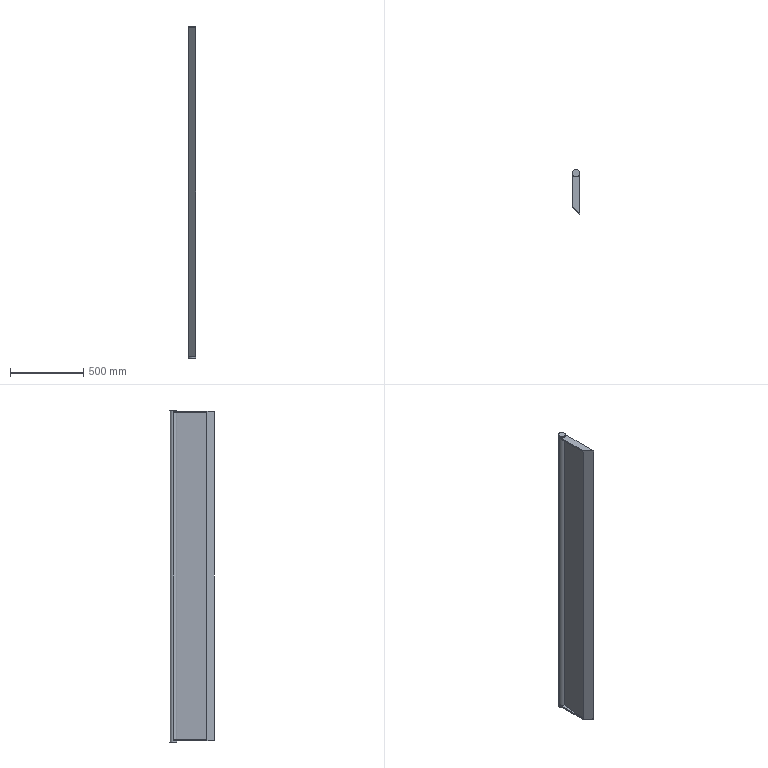Part | SolidWorks | 1 solid | 20 faces | box 50 x 305 x 2270 mm | volume 21360963 mm3 | plane 16 | cylinder 4 | commonest cylinder face diameters 50 x4
STEP:
#1=CARTESIAN_POINT('',(639.337,-63.085,2260.));
#2=VERTEX_POINT('',#1);
#3=CARTESIAN_POINT('',(589.337,-63.085,2260.));
#4=VERTEX_POINT('',#3);
#5=CARTESIAN_POINT('',(614.337,-63.085,2260.));
#6=DIRECTION('',(0.,0.,1.));
#7=DIRECTION('',(1.,0.,0.));
#8=AXIS2_PLACEMENT_3D('',#5,#6,#7);
#9=CIRCLE('',#8,25.);
#10=EDGE_CURVE('',#2,#4,#9,.T.);
#11=ORIENTED_EDGE('',*,*,#10,.F.);
#12=CARTESIAN_POINT('',(639.337,-63.085,2250.));
#13=VERTEX_POINT('',#12);
#14=CARTESIAN_POINT('',(639.337,-63.085,2260.));
#15=DIRECTION('',(0.,0.,-1.));
#16=VECTOR('',#15,1000.);
#17=LINE('',#14,#16);
#18=EDGE_CURVE('',#2,#13,#17,.T.);
#19=ORIENTED_EDGE('',*,*,#18,.T.);
#20=CARTESIAN_POINT('',(639.337,-63.085,2240.));
#21=VERTEX_POINT('',#20);
#22=CARTESIAN_POINT('',(639.337,-63.085,2250.));
#23=DIRECTION('',(0.,0.,-1.));
#24=VECTOR('',#23,1000.);
#25=LINE('',#22,#24);
#26=EDGE_CURVE('',#13,#21,#25,.T.);
#27=ORIENTED_EDGE('',*,*,#26,.T.);
#28=CARTESIAN_POINT('',(639.337,-63.085,10.));
#29=VERTEX_POINT('',#28);
#30=CARTESIAN_POINT('',(639.337,-63.085,2240.));
#31=DIRECTION('',(0.,0.,-1.));
#32=VECTOR('',#31,1000.);
#33=LINE('',#30,#32);
#34=EDGE_CURVE('',#21,#29,#33,.T.);
#35=ORIENTED_EDGE('',*,*,#34,.T.);
#36=CARTESIAN_POINT('',(639.337,-63.085,0.));
#37=VERTEX_POINT('',#36);
#38=CARTESIAN_POINT('',(639.337,-63.085,2250.));
#39=DIRECTION('',(0.,0.,-1.));
#40=VECTOR('',#39,1000.);
#41=LINE('',#38,#40);
#42=EDGE_CURVE('',#29,#37,#41,.T.);
#43=ORIENTED_EDGE('',*,*,#42,.T.);
#44=CARTESIAN_POINT('',(639.337,-63.085,-10.));
#45=VERTEX_POINT('',#44);
#46=CARTESIAN_POINT('',(639.337,-63.085,2260.));
#47=DIRECTION('',(0.,0.,-1.));
#48=VECTOR('',#47,1000.);
#49=LINE('',#46,#48);
#50=EDGE_CURVE('',#37,#45,#49,.T.);
#51=ORIENTED_EDGE('',*,*,#50,.T.);
#52=CARTESIAN_POINT('',(589.337,-63.085,-10.));
#53=VERTEX_POINT('',#52);
#54=CARTESIAN_POINT('',(614.337,-63.085,-10.));
#55=DIRECTION('',(0.,0.,1.));
#56=DIRECTION('',(1.,0.,0.));
#57=AXIS2_PLACEMENT_3D('',#54,#55,#56);
#58=CIRCLE('',#57,25.);
#59=EDGE_CURVE('',#45,#53,#58,.T.);
#60=ORIENTED_EDGE('',*,*,#59,.T.);
#61=CARTESIAN_POINT('',(589.337,-63.085,0.));
#62=VERTEX_POINT('',#61);
#63=CARTESIAN_POINT('',(589.337,-63.085,2260.));
#64=DIRECTION('',(0.,0.,-1.));
#65=VECTOR('',#64,1000.);
#66=LINE('',#63,#65);
#67=EDGE_CURVE('',#62,#53,#66,.T.);
#68=ORIENTED_EDGE('',*,*,#67,.F.);
#69=CARTESIAN_POINT('',(589.337,-63.085,10.));
#70=VERTEX_POINT('',#69);
#71=CARTESIAN_POINT('',(589.337,-63.085,2250.));
#72=DIRECTION('',(0.,0.,-1.));
#73=VECTOR('',#72,1000.);
#74=LINE('',#71,#73);
#75=EDGE_CURVE('',#70,#62,#74,.T.);
#76=ORIENTED_EDGE('',*,*,#75,.F.);
#77=CARTESIAN_POINT('',(589.337,-63.085,2240.));
#78=VERTEX_POINT('',#77);
#79=CARTESIAN_POINT('',(589.337,-63.085,2260.));
#80=DIRECTION('',(0.,0.,-1.));
#81=VECTOR('',#80,1000.);
#82=LINE('',#79,#81);
#83=EDGE_CURVE('',#78,#70,#82,.T.);
#84=ORIENTED_EDGE('',*,*,#83,.F.);
#85=CARTESIAN_POINT('',(589.337,-63.085,2250.));
#86=VERTEX_POINT('',#85);
#87=CARTESIAN_POINT('',(589.337,-63.085,2250.));
#88=DIRECTION('',(0.,0.,-1.));
#89=VECTOR('',#88,1000.);
#90=LINE('',#87,#89);
#91=EDGE_CURVE('',#86,#78,#90,.T.);
#92=ORIENTED_EDGE('',*,*,#91,.F.);
#93=CARTESIAN_POINT('',(589.337,-63.085,2260.));
#94=DIRECTION('',(0.,0.,-1.));
#95=VECTOR('',#94,1000.);
#96=LINE('',#93,#95);
#97=EDGE_CURVE('',#4,#86,#96,.T.);
#98=ORIENTED_EDGE('',*,*,#97,.F.);
#99=EDGE_LOOP('',(#11,#19,#27,#35,#43,#51,#60,#68,#76,#84,#92,#98));
#100=FACE_OUTER_BOUND('',#99,.T.);
#101=CARTESIAN_POINT('',(614.337,-63.085,2260.));
#102=DIRECTION('',(0.,0.,-1.));
#103=DIRECTION('',(-1.,0.,0.));
#104=AXIS2_PLACEMENT_3D('',#101,#102,#103);
#105=CYLINDRICAL_SURFACE('',#104,25.);
#106=ADVANCED_FACE('',(#100),#105,.T.);
#107=ORIENTED_EDGE('',*,*,#18,.F.);
#108=CARTESIAN_POINT('',(614.337,-63.085,2260.));
#109=DIRECTION('',(0.,0.,1.));
#110=DIRECTION('',(1.,0.,0.));
#111=AXIS2_PLACEMENT_3D('',#108,#109,#110);
#112=CIRCLE('',#111,25.);
#113=EDGE_CURVE('',#4,#2,#112,.T.);
#114=ORIENTED_EDGE('',*,*,#113,.F.);
#115=ORIENTED_EDGE('',*,*,#97,.T.);
#116=CARTESIAN_POINT('',(614.337,-63.085,2250.));
#117=DIRECTION('',(0.,0.,-1.));
#118=DIRECTION('',(-1.,0.,0.));
#119=AXIS2_PLACEMENT_3D('',#116,#117,#118);
#120=CIRCLE('',#119,25.);
#121=EDGE_CURVE('',#13,#86,#120,.T.);
#122=ORIENTED_EDGE('',*,*,#121,.F.);
#123=EDGE_LOOP('',(#107,#114,#115,#122));
#124=FACE_OUTER_BOUND('',#123,.T.);
#125=CARTESIAN_POINT('',(614.337,-63.085,2260.));
#126=DIRECTION('',(0.,0.,-1.));
#127=DIRECTION('',(-1.,0.,0.));
#128=AXIS2_PLACEMENT_3D('',#125,#126,#127);
#129=CYLINDRICAL_SURFACE('',#128,25.);
#130=ADVANCED_FACE('',(#124),#129,.T.);
#131=CARTESIAN_POINT('',(611.635,-87.939,2240.));
#132=VERTEX_POINT('',#131);
#133=CARTESIAN_POINT('',(614.337,-63.085,2240.));
#134=DIRECTION('',(0.,0.,1.));
#135=DIRECTION('',(1.,0.,0.));
#136=AXIS2_PLACEMENT_3D('',#133,#134,#135);
#137=CIRCLE('',#136,25.);
#138=EDGE_CURVE('',#78,#132,#137,.T.);
#139=ORIENTED_EDGE('',*,*,#138,.F.);
#140=ORIENTED_EDGE('',*,*,#83,.T.);
#141=CARTESIAN_POINT('',(611.635,-87.939,10.));
#142=VERTEX_POINT('',#141);
#143=CARTESIAN_POINT('',(614.337,-63.085,10.));
#144=DIRECTION('',(0.,0.,1.));
#145=DIRECTION('',(1.,0.,0.));
#146=AXIS2_PLACEMENT_3D('',#143,#144,#145);
#147=CIRCLE('',#146,25.);
#148=EDGE_CURVE('',#70,#142,#147,.T.);
#149=ORIENTED_EDGE('',*,*,#148,.T.);
#150=CARTESIAN_POINT('',(611.635,-87.939,2240.));
#151=DIRECTION('',(0.,0.,-1.));
#152=VECTOR('',#151,1000.);
#153=LINE('',#150,#152);
#154=EDGE_CURVE('',#132,#142,#153,.T.);
#155=ORIENTED_EDGE('',*,*,#154,.F.);
#156=EDGE_LOOP('',(#139,#140,#149,#155));
#157=FACE_OUTER_BOUND('',#156,.T.);
#158=CARTESIAN_POINT('',(614.337,-63.085,2260.));
#159=DIRECTION('',(0.,0.,-1.));
#160=DIRECTION('',(-1.,0.,0.));
#161=AXIS2_PLACEMENT_3D('',#158,#159,#160);
#162=CYLINDRICAL_SURFACE('',#161,25.);
#163=ADVANCED_FACE('',(#157),#162,.T.);
#164=CARTESIAN_POINT('',(589.337,-293.085,10.));
#165=VERTEX_POINT('',#164);
#166=CARTESIAN_POINT('',(589.337,0.,10.));
#167=DIRECTION('',(0.,-1.,0.));
#168=VECTOR('',#167,1000.);
#169=LINE('',#166,#168);
#170=EDGE_CURVE('',#70,#165,#169,.T.);
#171=ORIENTED_EDGE('',*,*,#170,.F.);
#172=ORIENTED_EDGE('',*,*,#75,.T.);
#173=CARTESIAN_POINT('',(589.337,-293.085,0.));
#174=VERTEX_POINT('',#173);
#175=CARTESIAN_POINT('',(589.337,-293.085,0.));
#176=DIRECTION('',(0.,-1.,0.));
#177=VECTOR('',#176,1000.);
#178=LINE('',#175,#177);
#179=EDGE_CURVE('',#62,#174,#178,.T.);
#180=ORIENTED_EDGE('',*,*,#179,.T.);
#181=CARTESIAN_POINT('',(589.337,-293.085,2250.));
#182=DIRECTION('',(0.,0.,-1.));
#183=VECTOR('',#182,1000.);
#184=LINE('',#181,#183);
#185=EDGE_CURVE('',#165,#174,#184,.T.);
#186=ORIENTED_EDGE('',*,*,#185,.F.);
#187=EDGE_LOOP('',(#171,#172,#180,#186));
#188=FACE_OUTER_BOUND('',#187,.T.);
#189=CARTESIAN_POINT('',(589.337,-293.085,2250.));
#190=DIRECTION('',(1.,0.,0.));
#191=DIRECTION('',(0.,1.,0.));
#192=AXIS2_PLACEMENT_3D('',#189,#190,#191);
#193=PLANE('',#192);
#194=ADVANCED_FACE('',(#188),#193,.F.);
#195=CARTESIAN_POINT('',(639.337,-343.085,2240.));
#196=VERTEX_POINT('',#195);
#197=CARTESIAN_POINT('',(639.337,-63.085,2240.));
#198=DIRECTION('',(0.,1.,0.));
#199=VECTOR('',#198,1000.);
#200=LINE('',#197,#199);
#201=EDGE_CURVE('',#196,#21,#200,.T.);
#202=ORIENTED_EDGE('',*,*,#201,.T.);
#203=ORIENTED_EDGE('',*,*,#26,.F.);
#204=CARTESIAN_POINT('',(639.337,-343.085,2250.));
#205=VERTEX_POINT('',#204);
#206=CARTESIAN_POINT('',(639.337,-283.085,2250.));
#207=DIRECTION('',(0.,1.,0.));
#208=VECTOR('',#207,1000.);
#209=LINE('',#206,#208);
#210=EDGE_CURVE('',#205,#13,#209,.T.);
#211=ORIENTED_EDGE('',*,*,#210,.F.);
#212=CARTESIAN_POINT('',(639.337,-343.085,2250.));
#213=DIRECTION('',(0.,0.,-1.));
#214=VECTOR('',#213,1000.);
#215=LINE('',#212,#214);
#216=EDGE_CURVE('',#205,#196,#215,.T.);
#217=ORIENTED_EDGE('',*,*,#216,.T.);
#218=EDGE_LOOP('',(#202,#203,#211,#217));
#219=FACE_OUTER_BOUND('',#218,.T.);
#220=CARTESIAN_POINT('',(639.337,-63.085,2250.));
#221=DIRECTION('',(-1.,0.,0.));
#222=DIRECTION('',(0.,0.,1.));
#223=AXIS2_PLACEMENT_3D('',#220,#221,#222);
#224=PLANE('',#223);
#225=ADVANCED_FACE('',(#219),#224,.F.);
#226=ORIENTED_EDGE('',*,*,#50,.F.);
#227=CARTESIAN_POINT('',(614.337,-63.085,0.));
#228=DIRECTION('',(0.,0.,-1.));
#229=DIRECTION('',(-1.,0.,0.));
#230=AXIS2_PLACEMENT_3D('',#227,#228,#229);
#231=CIRCLE('',#230,25.);
#232=EDGE_CURVE('',#37,#62,#231,.T.);
#233=ORIENTED_EDGE('',*,*,#232,.T.);
#234=ORIENTED_EDGE('',*,*,#67,.T.);
#235=CARTESIAN_POINT('',(614.337,-63.085,-10.));
#236=DIRECTION('',(0.,0.,1.));
#237=DIRECTION('',(1.,0.,0.));
#238=AXIS2_PLACEMENT_3D('',#235,#236,#237);
#239=CIRCLE('',#238,25.);
#240=EDGE_CURVE('',#53,#45,#239,.T.);
#241=ORIENTED_EDGE('',*,*,#240,.T.);
#242=EDGE_LOOP('',(#226,#233,#234,#241));
#243=FACE_OUTER_BOUND('',#242,.T.);
#244=CARTESIAN_POINT('',(614.337,-63.085,2260.));
#245=DIRECTION('',(0.,0.,-1.));
#246=DIRECTION('',(-1.,0.,0.));
#247=AXIS2_PLACEMENT_3D('',#244,#245,#246);
#248=CYLINDRICAL_SURFACE('',#247,25.);
#249=ADVANCED_FACE('',(#243),#248,.T.);
#250=ORIENTED_EDGE('',*,*,#113,.T.);
#251=ORIENTED_EDGE('',*,*,#10,.T.);
#252=EDGE_LOOP('',(#250,#251));
#253=FACE_OUTER_BOUND('',#252,.T.);
#254=CARTESIAN_POINT('',(614.337,-63.085,2260.));
#255=DIRECTION('',(0.,0.,1.));
#256=DIRECTION('',(1.,0.,0.));
#257=AXIS2_PLACEMENT_3D('',#254,#255,#256);
#258=PLANE('',#257);
#259=ADVANCED_FACE('',(#253),#258,.T.);
#260=ORIENTED_EDGE('',*,*,#240,.F.);
#261=ORIENTED_EDGE('',*,*,#59,.F.);
#262=EDGE_LOOP('',(#260,#261));
#263=FACE_OUTER_BOUND('',#262,.T.);
#264=CARTESIAN_POINT('',(614.337,-63.085,-10.));
#265=DIRECTION('',(0.,0.,1.));
#266=DIRECTION('',(1.,0.,0.));
#267=AXIS2_PLACEMENT_3D('',#264,#265,#266);
#268=PLANE('',#267);
#269=ADVANCED_FACE('',(#263),#268,.F.);
#270=ORIENTED_EDGE('',*,*,#91,.T.);
#271=CARTESIAN_POINT('',(589.337,-293.085,2240.));
#272=VERTEX_POINT('',#271);
#273=CARTESIAN_POINT('',(589.337,0.,2240.));
#274=DIRECTION('',(0.,-1.,0.));
#275=VECTOR('',#274,1000.);
#276=LINE('',#273,#275);
#277=EDGE_CURVE('',#78,#272,#276,.T.);
#278=ORIENTED_EDGE('',*,*,#277,.T.);
#279=CARTESIAN_POINT('',(589.337,-293.085,2250.));
#280=VERTEX_POINT('',#279);
#281=CARTESIAN_POINT('',(589.337,-293.085,2250.));
#282=DIRECTION('',(0.,0.,-1.));
#283=VECTOR('',#282,1000.);
#284=LINE('',#281,#283);
#285=EDGE_CURVE('',#280,#272,#284,.T.);
#286=ORIENTED_EDGE('',*,*,#285,.F.);
#287=CARTESIAN_POINT('',(589.337,-293.085,2250.));
#288=DIRECTION('',(0.,-1.,0.));
#289=VECTOR('',#288,1000.);
#290=LINE('',#287,#289);
#291=EDGE_CURVE('',#86,#280,#290,.T.);
#292=ORIENTED_EDGE('',*,*,#291,.F.);
#293=EDGE_LOOP('',(#270,#278,#286,#292));
#294=FACE_OUTER_BOUND('',#293,.T.);
#295=CARTESIAN_POINT('',(589.337,-293.085,2250.));
#296=DIRECTION('',(1.,0.,0.));
#297=DIRECTION('',(0.,1.,0.));
#298=AXIS2_PLACEMENT_3D('',#295,#296,#297);
#299=PLANE('',#298);
#300=ADVANCED_FACE('',(#294),#299,.F.);
#301=CARTESIAN_POINT('',(639.337,-343.085,0.));
#302=VERTEX_POINT('',#301);
#303=CARTESIAN_POINT('',(639.337,-343.085,0.));
#304=DIRECTION('',(0.7071,-0.7071,0.));
#305=VECTOR('',#304,1000.);
#306=LINE('',#303,#305);
#307=EDGE_CURVE('',#174,#302,#306,.T.);
#308=ORIENTED_EDGE('',*,*,#307,.T.);
#309=CARTESIAN_POINT('',(639.337,-343.085,10.));
#310=VERTEX_POINT('',#309);
#311=CARTESIAN_POINT('',(639.337,-343.085,2250.));
#312=DIRECTION('',(0.,0.,-1.));
#313=VECTOR('',#312,1000.);
#314=LINE('',#311,#313);
#315=EDGE_CURVE('',#310,#302,#314,.T.);
#316=ORIENTED_EDGE('',*,*,#315,.F.);
#317=CARTESIAN_POINT('',(639.337,-343.085,2240.));
#318=DIRECTION('',(0.,0.,-1.));
#319=VECTOR('',#318,1000.);
#320=LINE('',#317,#319);
#321=EDGE_CURVE('',#196,#310,#320,.T.);
#322=ORIENTED_EDGE('',*,*,#321,.F.);
#323=ORIENTED_EDGE('',*,*,#216,.F.);
#324=CARTESIAN_POINT('',(639.337,-343.085,2250.));
#325=DIRECTION('',(0.7071,-0.7071,0.));
#326=VECTOR('',#325,1000.);
#327=LINE('',#324,#326);
#328=EDGE_CURVE('',#280,#205,#327,.T.);
#329=ORIENTED_EDGE('',*,*,#328,.F.);
#330=ORIENTED_EDGE('',*,*,#285,.T.);
#331=CARTESIAN_POINT('',(589.337,-293.085,2240.));
#332=DIRECTION('',(0.,0.,-1.));
#333=VECTOR('',#332,1000.);
#334=LINE('',#331,#333);
#335=EDGE_CURVE('',#272,#165,#334,.T.);
#336=ORIENTED_EDGE('',*,*,#335,.T.);
#337=ORIENTED_EDGE('',*,*,#185,.T.);
#338=EDGE_LOOP('',(#308,#316,#322,#323,#329,#330,#336,#337));
#339=FACE_OUTER_BOUND('',#338,.T.);
#340=CARTESIAN_POINT('',(639.337,-343.085,2250.));
#341=DIRECTION('',(0.7071,0.7071,0.));
#342=DIRECTION('',(-0.7071,0.7071,0.));
#343=AXIS2_PLACEMENT_3D('',#340,#341,#342);
#344=PLANE('',#343);
#345=ADVANCED_FACE('',(#339),#344,.F.);
#346=ORIENTED_EDGE('',*,*,#42,.F.);
#347=CARTESIAN_POINT('',(639.337,-63.085,10.));
#348=DIRECTION('',(0.,1.,0.));
#349=VECTOR('',#348,1000.);
#350=LINE('',#347,#349);
#351=EDGE_CURVE('',#310,#29,#350,.T.);
#352=ORIENTED_EDGE('',*,*,#351,.F.);
#353=ORIENTED_EDGE('',*,*,#315,.T.);
#354=CARTESIAN_POINT('',(639.337,-63.085,0.));
#355=DIRECTION('',(0.,1.,0.));
#356=VECTOR('',#355,1000.);
#357=LINE('',#354,#356);
#358=EDGE_CURVE('',#302,#37,#357,.T.);
#359=ORIENTED_EDGE('',*,*,#358,.T.);
#360=EDGE_LOOP('',(#346,#352,#353,#359));
#361=FACE_OUTER_BOUND('',#360,.T.);
#362=CARTESIAN_POINT('',(639.337,-63.085,2250.));
#363=DIRECTION('',(-1.,0.,0.));
#364=DIRECTION('',(0.,0.,1.));
#365=AXIS2_PLACEMENT_3D('',#362,#363,#364);
#366=PLANE('',#365);
#367=ADVANCED_FACE('',(#361),#366,.F.);
#368=ORIENTED_EDGE('',*,*,#210,.T.);
#369=ORIENTED_EDGE('',*,*,#121,.T.);
#370=ORIENTED_EDGE('',*,*,#291,.T.);
#371=ORIENTED_EDGE('',*,*,#328,.T.);
#372=EDGE_LOOP('',(#368,#369,#370,#371));
#373=FACE_OUTER_BOUND('',#372,.T.);
#374=CARTESIAN_POINT('',(0.,0.,2250.));
#375=DIRECTION('',(0.,0.,-1.));
#376=DIRECTION('',(-1.,0.,0.));
#377=AXIS2_PLACEMENT_3D('',#374,#375,#376);
#378=PLANE('',#377);
#379=ADVANCED_FACE('',(#373),#378,.F.);
#380=ORIENTED_EDGE('',*,*,#232,.F.);
#381=ORIENTED_EDGE('',*,*,#358,.F.);
#382=ORIENTED_EDGE('',*,*,#307,.F.);
#383=ORIENTED_EDGE('',*,*,#179,.F.);
#384=EDGE_LOOP('',(#380,#381,#382,#383));
#385=FACE_OUTER_BOUND('',#384,.T.);
#386=CARTESIAN_POINT('',(0.,0.,0.));
#387=DIRECTION('',(0.,0.,-1.));
#388=DIRECTION('',(-1.,0.,0.));
#389=AXIS2_PLACEMENT_3D('',#386,#387,#388);
#390=PLANE('',#389);
#391=ADVANCED_FACE('',(#385),#390,.T.);
#392=CARTESIAN_POINT('',(625.939,-293.085,10.));
#393=VERTEX_POINT('',#392);
#394=CARTESIAN_POINT('',(625.939,-293.085,10.));
#395=DIRECTION('',(-0.05815,-0.9983,0.));
#396=VECTOR('',#395,1000.);
#397=LINE('',#394,#396);
#398=EDGE_CURVE('',#29,#393,#397,.T.);
#399=ORIENTED_EDGE('',*,*,#398,.F.);
#400=ORIENTED_EDGE('',*,*,#34,.F.);
#401=CARTESIAN_POINT('',(625.939,-293.085,2240.));
#402=VERTEX_POINT('',#401);
#403=CARTESIAN_POINT('',(625.939,-293.085,2240.));
#404=DIRECTION('',(-0.05815,-0.9983,0.));
#405=VECTOR('',#404,1000.);
#406=LINE('',#403,#405);
#407=EDGE_CURVE('',#21,#402,#406,.T.);
#408=ORIENTED_EDGE('',*,*,#407,.T.);
#409=CARTESIAN_POINT('',(625.939,-293.085,2240.));
#410=DIRECTION('',(0.,0.,-1.));
#411=VECTOR('',#410,1000.);
#412=LINE('',#409,#411);
#413=EDGE_CURVE('',#402,#393,#412,.T.);
#414=ORIENTED_EDGE('',*,*,#413,.T.);
#415=EDGE_LOOP('',(#399,#400,#408,#414));
#416=FACE_OUTER_BOUND('',#415,.T.);
#417=CARTESIAN_POINT('',(625.939,-293.085,2240.));
#418=DIRECTION('',(0.9983,-0.05815,0.));
#419=DIRECTION('',(0.05815,0.9983,0.));
#420=AXIS2_PLACEMENT_3D('',#417,#418,#419);
#421=PLANE('',#420);
#422=ADVANCED_FACE('',(#416),#421,.T.);
#423=CARTESIAN_POINT('',(639.337,-343.085,10.));
#424=DIRECTION('',(0.2588,-0.9659,0.));
#425=VECTOR('',#424,1000.);
#426=LINE('',#423,#425);
#427=EDGE_CURVE('',#393,#310,#426,.T.);
#428=ORIENTED_EDGE('',*,*,#427,.F.);
#429=ORIENTED_EDGE('',*,*,#413,.F.);
#430=CARTESIAN_POINT('',(639.337,-343.085,2240.));
#431=DIRECTION('',(0.2588,-0.9659,0.));
#432=VECTOR('',#431,1000.);
#433=LINE('',#430,#432);
#434=EDGE_CURVE('',#402,#196,#433,.T.);
#435=ORIENTED_EDGE('',*,*,#434,.T.);
#436=ORIENTED_EDGE('',*,*,#321,.T.);
#437=EDGE_LOOP('',(#428,#429,#435,#436));
#438=FACE_OUTER_BOUND('',#437,.T.);
#439=CARTESIAN_POINT('',(639.337,-343.085,2240.));
#440=DIRECTION('',(0.9659,0.2588,0.));
#441=DIRECTION('',(-0.2588,0.9659,0.));
#442=AXIS2_PLACEMENT_3D('',#439,#440,#441);
#443=PLANE('',#442);
#444=ADVANCED_FACE('',(#438),#443,.T.);
#445=ORIENTED_EDGE('',*,*,#201,.F.);
#446=ORIENTED_EDGE('',*,*,#434,.F.);
#447=ORIENTED_EDGE('',*,*,#407,.F.);
#448=EDGE_LOOP('',(#445,#446,#447));
#449=FACE_OUTER_BOUND('',#448,.T.);
#450=CARTESIAN_POINT('',(0.,0.,2240.));
#451=DIRECTION('',(0.,0.,-1.));
#452=DIRECTION('',(-1.,0.,0.));
#453=AXIS2_PLACEMENT_3D('',#450,#451,#452);
#454=PLANE('',#453);
#455=ADVANCED_FACE('',(#449),#454,.T.);
#456=ORIENTED_EDGE('',*,*,#351,.T.);
#457=ORIENTED_EDGE('',*,*,#398,.T.);
#458=ORIENTED_EDGE('',*,*,#427,.T.);
#459=EDGE_LOOP('',(#456,#457,#458));
#460=FACE_OUTER_BOUND('',#459,.T.);
#461=CARTESIAN_POINT('',(0.,0.,10.));
#462=DIRECTION('',(0.,0.,-1.));
#463=DIRECTION('',(-1.,0.,0.));
#464=AXIS2_PLACEMENT_3D('',#461,#462,#463);
#465=PLANE('',#464);
#466=ADVANCED_FACE('',(#460),#465,.F.);
#467=CARTESIAN_POINT('',(613.94,-66.733,10.));
#468=DIRECTION('',(0.1081,0.9941,0.));
#469=VECTOR('',#468,1000.);
#470=LINE('',#467,#469);
#471=EDGE_CURVE('',#165,#142,#470,.T.);
#472=ORIENTED_EDGE('',*,*,#471,.F.);
#473=ORIENTED_EDGE('',*,*,#335,.F.);
#474=CARTESIAN_POINT('',(613.94,-66.733,2240.));
#475=DIRECTION('',(0.1081,0.9941,0.));
#476=VECTOR('',#475,1000.);
#477=LINE('',#474,#476);
#478=EDGE_CURVE('',#272,#132,#477,.T.);
#479=ORIENTED_EDGE('',*,*,#478,.T.);
#480=ORIENTED_EDGE('',*,*,#154,.T.);
#481=EDGE_LOOP('',(#472,#473,#479,#480));
#482=FACE_OUTER_BOUND('',#481,.T.);
#483=CARTESIAN_POINT('',(613.94,-66.733,2240.));
#484=DIRECTION('',(-0.9941,0.1081,0.));
#485=DIRECTION('',(-0.1081,-0.9941,0.));
#486=AXIS2_PLACEMENT_3D('',#483,#484,#485);
#487=PLANE('',#486);
#488=ADVANCED_FACE('',(#482),#487,.T.);
#489=ORIENTED_EDGE('',*,*,#138,.T.);
#490=ORIENTED_EDGE('',*,*,#478,.F.);
#491=ORIENTED_EDGE('',*,*,#277,.F.);
#492=EDGE_LOOP('',(#489,#490,#491));
#493=FACE_OUTER_BOUND('',#492,.T.);
#494=CARTESIAN_POINT('',(0.,0.,2240.));
#495=DIRECTION('',(0.,0.,1.));
#496=DIRECTION('',(1.,0.,0.));
#497=AXIS2_PLACEMENT_3D('',#494,#495,#496);
#498=PLANE('',#497);
#499=ADVANCED_FACE('',(#493),#498,.F.);
#500=ORIENTED_EDGE('',*,*,#148,.F.);
#501=ORIENTED_EDGE('',*,*,#170,.T.);
#502=ORIENTED_EDGE('',*,*,#471,.T.);
#503=EDGE_LOOP('',(#500,#501,#502));
#504=FACE_OUTER_BOUND('',#503,.T.);
#505=CARTESIAN_POINT('',(0.,0.,10.));
#506=DIRECTION('',(0.,0.,1.));
#507=DIRECTION('',(1.,0.,0.));
#508=AXIS2_PLACEMENT_3D('',#505,#506,#507);
#509=PLANE('',#508);
#510=ADVANCED_FACE('',(#504),#509,.T.);
#511=CLOSED_SHELL('',(#106,#130,#163,#194,#225,#249,#259,#269,#300,#345,#367,#379,#391,#422,#444,#455,#466,#488,#499,#510));
#512=MANIFOLD_SOLID_BREP('',#511);
#513=CARTESIAN_POINT('',(0.,0.,0.));
#514=DIRECTION('',(0.,0.,1.));
#515=DIRECTION('',(1.,0.,0.));
#516=AXIS2_PLACEMENT_3D('',#513,#514,#515);
#517=(LENGTH_UNIT()NAMED_UNIT(*)SI_UNIT(.MILLI.,.METRE.));
#518=UNCERTAINTY_MEASURE_WITH_UNIT(LENGTH_MEASURE(0.00001),#517,'','');
#519=(NAMED_UNIT(*)PLANE_ANGLE_UNIT()SI_UNIT($,.RADIAN.));
#520=(NAMED_UNIT(*)SI_UNIT($,.STERADIAN.)SOLID_ANGLE_UNIT());
#521=(GEOMETRIC_REPRESENTATION_CONTEXT(3)GLOBAL_UNCERTAINTY_ASSIGNED_CONTEXT((#518))GLOBAL_UNIT_ASSIGNED_CONTEXT((#517,#519,#520))REPRESENTATION_CONTEXT('',''));
#522=ADVANCED_BREP_SHAPE_REPRESENTATION('',(#512,#516),#521);